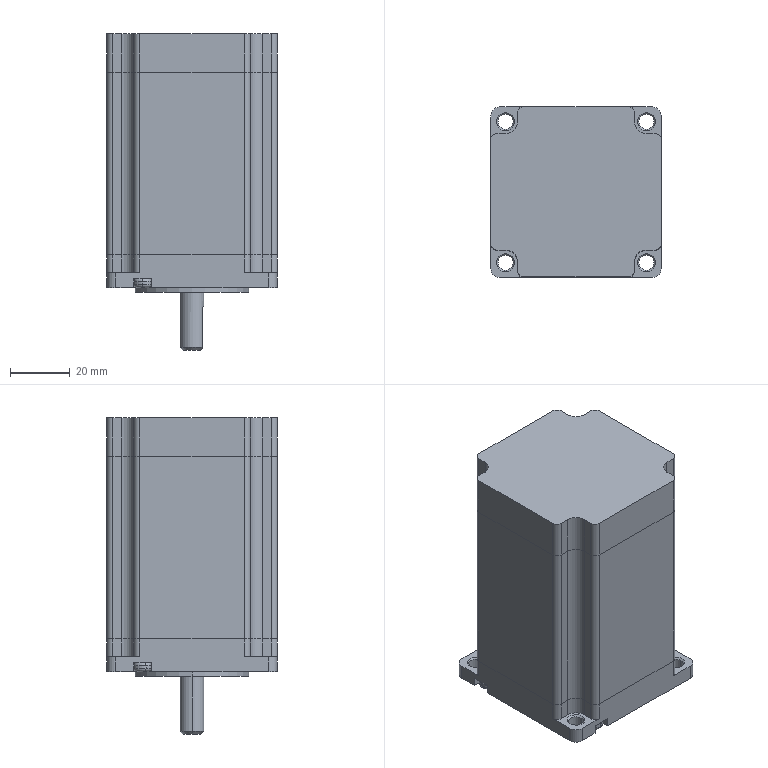Part | SolidWorks | 8 solids | 273 faces | box 57 x 57 x 106 mm | volume 252225 mm3 | plane 160 | cylinder 83 | torus 20 | cone 10 | commonest cylinder face diameters 4 x24 6 x19 8 x16 3 x8 5 x8 10 x6